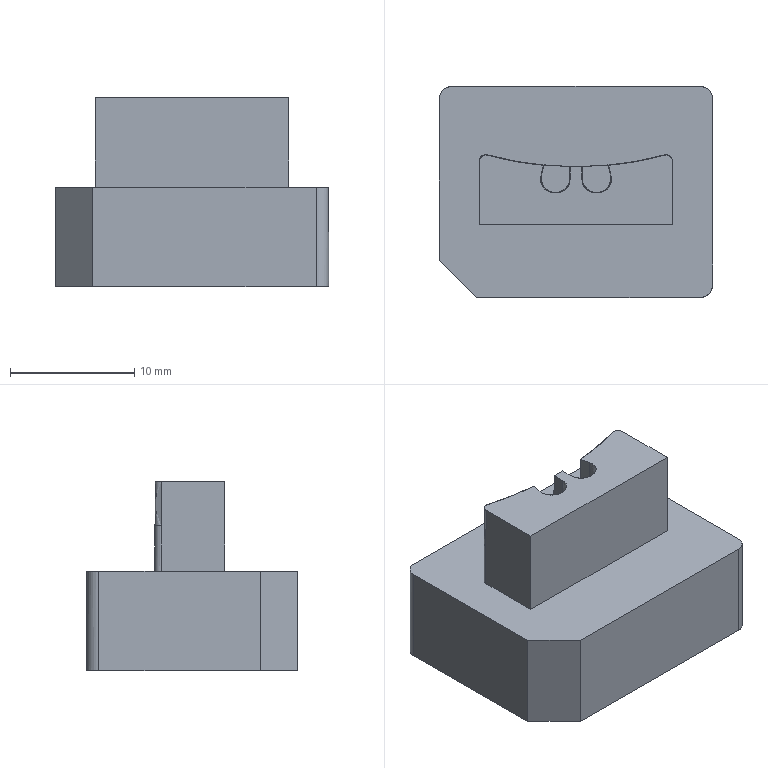NC program | PowerMill | posted by the shop | part box 22 x 17 x 15.232 mm
Lines 2761 to 5582 of 87032, first 2527 of 2822 lines:
( TOOL ID   D3C_1_1 )
( TOOL DIA. 3. TIP RAD 0 LENGTH 62.4 )
( Z = -7.32 )
T15 M6
T27
G91 G28 Z0
G0 G90 G54
M08
S18000 M3
X0 Y0 M8
G43 Z9.812 H15
X1.43 Y-5.074
Z.863
G1 Z-.337 F3000
X1.438 Y-5.057 F5000
G3 X1.361 Y-4.825 I-.155 J.077
G1 X0 Y-4.144
X-7.809
X-8.232 Y-4.074
X-8.399 Y-4.01
X-8.654 Y-3.864
X-8.949 Y-3.588
X-9.076 Y-3.409
X-9.194 Y-3.166
X-9.289 Y-2.744
X-9.294 Y-2.322
Y2.322
X-9.268 Y2.744
X-9.167 Y3.166
X-8.95 Y3.588
X-8.654 Y3.936
X-8.232 Y4.236
X-7.809 Y4.401
X-7.387 Y4.478
X-6.965 Y4.452
X-5.277 Y4.065
X-4.01 Y3.835
X-2.21 Y3.588
X-1.9 Y3.456
X-1.578 Y3.201
X-1.494 Y3.168
X-1.406 Y3.19
X-1.055 Y3.407
X-.633 Y3.515
X.633
X1.055 Y3.407
X1.406 Y3.19
X1.482 Y3.168
X1.558 Y3.189
X1.578 Y3.2
X1.9 Y3.456
X2.21 Y3.588
X3.588 Y3.775
X5.277 Y4.065
X6.826 Y4.432
X7.387 Y4.478
X7.693 Y4.432
X8.232 Y4.236
X8.569 Y4.01
X8.95 Y3.588
X9.162 Y3.166
X9.259 Y2.744
X9.294 Y2.322
Y-2.322
X9.289 Y-2.744
X9.194 Y-3.166
X9.076 Y-3.409
X8.949 Y-3.588
X8.654 Y-3.864
X8.399 Y-4.01
X8.232 Y-4.074
X7.809 Y-4.144
X0
X1.43 Y-5.074 Z-.485
X1.438 Y-5.057
G3 X1.361 Y-4.825 I-.155 J.077
G1 X0 Y-4.144
X-7.809
X-8.232 Y-4.074
X-8.399 Y-4.01
X-8.654 Y-3.864
X-8.949 Y-3.588
X-9.076 Y-3.409
X-9.194 Y-3.166
X-9.289 Y-2.744
X-9.294 Y-2.322
Y2.322
X-9.268 Y2.744
X-9.168 Y3.166
X-8.95 Y3.588
X-8.654 Y3.937
X-8.232 Y4.242
X-7.809 Y4.404
X-7.387 Y4.481
X-6.965 Y4.454
X-5.699 Y4.164
X-4.01 Y3.838
X-2.205 Y3.588
X-1.9 Y3.459
X-1.578 Y3.203
X-1.493 Y3.171
X-1.405 Y3.194
X-1.055 Y3.412
X-.633 Y3.52
X.633
X1.055 Y3.412
X1.405 Y3.194
X1.493 Y3.171
X1.578 Y3.203
X1.9 Y3.459
X2.205 Y3.588
X3.726 Y3.798
X3.728 Y3.799
X5.017 Y4.02
X5.277 Y4.067
X6.818 Y4.432
X7.387 Y4.481
X7.699 Y4.432
X8.232 Y4.242
X8.573 Y4.01
X8.95 Y3.588
X9.168 Y3.166
X9.261 Y2.744
X9.294 Y2.322
Y-2.322
X9.289 Y-2.744
X9.194 Y-3.166
X9.076 Y-3.409
X8.949 Y-3.588
X8.654 Y-3.864
X8.399 Y-4.01
X8.232 Y-4.074
X7.809 Y-4.144
X0
X1.43 Y-5.074 Z-.634
X1.438 Y-5.057
G3 X1.361 Y-4.825 I-.155 J.077
G1 X0 Y-4.144
X-7.809
X-8.232 Y-4.074
X-8.399 Y-4.01
X-8.654 Y-3.864
X-8.949 Y-3.588
X-9.076 Y-3.409
X-9.194 Y-3.166
X-9.289 Y-2.744
X-9.294 Y-2.322
Y2.322
X-9.268 Y2.744
X-9.168 Y3.166
X-8.95 Y3.588
X-8.654 Y3.938
X-8.232 Y4.243
X-7.809 Y4.408
X-7.387 Y4.483
X-6.965 Y4.456
X-5.699 Y4.165
X-4.01 Y3.839
X-2.322 Y3.619
X-2.265 Y3.597
X-2.205 Y3.588
X-1.955 Y3.483
X-1.9 Y3.462
X-1.578 Y3.206
X-1.493 Y3.174
X-1.405 Y3.196
X-1.055 Y3.416
X-.633 Y3.521
X.633
X1.055 Y3.416
X1.405 Y3.196
X1.493 Y3.174
X1.578 Y3.206
X1.9 Y3.462
X2.199 Y3.588
X3.772 Y3.806
X3.775 Y3.807
X4.862 Y3.994
X5.277 Y4.069
X6.812 Y4.432
X7.387 Y4.483
X7.703 Y4.432
X8.232 Y4.243
X8.574 Y4.01
X8.95 Y3.588
X9.168 Y3.166
X9.264 Y2.744
X9.294 Y2.322
Y-2.322
X9.289 Y-2.744
X9.194 Y-3.166
X9.076 Y-3.409
X8.949 Y-3.588
X8.654 Y-3.864
X8.399 Y-4.01
X8.232 Y-4.074
X7.809 Y-4.144
X0
X1.43 Y-5.074 Z-.782
X1.438 Y-5.057
G3 X1.361 Y-4.825 I-.155 J.077
G1 X0 Y-4.144
X-7.809
X-8.232 Y-4.074
X-8.399 Y-4.01
X-8.654 Y-3.864
X-8.949 Y-3.588
X-9.076 Y-3.409
X-9.194 Y-3.166
X-9.289 Y-2.744
X-9.294 Y-2.322
Y2.322
X-9.269 Y2.744
X-9.169 Y3.166
X-8.95 Y3.588
X-8.654 Y3.94
X-8.232 Y4.244
X-7.809 Y4.411
X-7.387 Y4.484
X-6.965 Y4.458
X-5.649 Y4.156
X-5.646 Y4.155
X-4.128 Y3.862
X-4.01 Y3.841
X-2.322 Y3.621
X-2.109 Y3.548
X-1.9 Y3.465
X-1.578 Y3.209
X-1.493 Y3.176
X-1.405 Y3.199
X-1.055 Y3.418
X-.633 Y3.523
X.633
X1.055 Y3.418
X1.405 Y3.199
X1.493 Y3.176
X1.578 Y3.209
X1.9 Y3.465
X2.194 Y3.588
X3.588 Y3.783
X5.277 Y4.07
X6.806 Y4.432
X7.387 Y4.484
X7.707 Y4.432
X8.232 Y4.244
X8.575 Y4.01
X8.95 Y3.588
X9.169 Y3.166
X9.266 Y2.744
X9.294 Y2.322
Y-2.322
X9.289 Y-2.744
X9.194 Y-3.166
X9.076 Y-3.409
X8.949 Y-3.588
X8.654 Y-3.864
X8.399 Y-4.01
X8.232 Y-4.074
X7.809 Y-4.144
X0
X1.43 Y-5.074 Z-.931
X1.438 Y-5.057
G3 X1.361 Y-4.825 I-.155 J.077
G1 X0 Y-4.144
X-7.809
X-8.232 Y-4.074
X-8.399 Y-4.01
X-8.654 Y-3.864
X-8.949 Y-3.588
X-9.076 Y-3.409
X-9.194 Y-3.166
X-9.289 Y-2.744
X-9.294 Y-2.322
Y2.322
X-9.269 Y2.744
X-9.169 Y3.166
X-8.95 Y3.588
X-8.654 Y3.941
X-8.232 Y4.246
X-7.809 Y4.412
X-7.387 Y4.486
X-6.965 Y4.46
X-5.608 Y4.148
X-4.246 Y3.885
X-4.01 Y3.842
X-2.322 Y3.622
X-2.244 Y3.593
X-2.205 Y3.588
X-2.054 Y3.524
X-1.9 Y3.467
X-1.577 Y3.211
X-1.493 Y3.179
X-1.405 Y3.201
X-1.055 Y3.419
X-.633 Y3.524
X.633
X1.055 Y3.419
X1.405 Y3.201
X1.492 Y3.179
X1.577 Y3.211
X1.9 Y3.467
X1.949 Y3.485
X1.952 Y3.487
X2.194 Y3.588
X2.26 Y3.598
X2.322 Y3.622
X3.588 Y3.784
X5.277 Y4.071
X6.8 Y4.432
X7.387 Y4.486
X7.71 Y4.432
X8.232 Y4.246
X8.576 Y4.01
X8.951 Y3.588
X9.169 Y3.166
X9.269 Y2.744
X9.294 Y2.322
Y-2.322
X9.289 Y-2.744
X9.194 Y-3.166
X9.076 Y-3.409
X8.949 Y-3.588
X8.654 Y-3.864
X8.399 Y-4.01
X8.232 Y-4.074
X7.809 Y-4.144
X0
X1.43 Y-5.074 Z-1.079
X1.438 Y-5.057
G3 X1.361 Y-4.825 I-.155 J.077
G1 X0 Y-4.144
X-7.809
X-8.232 Y-4.074
X-8.399 Y-4.01
X-8.654 Y-3.864
X-8.949 Y-3.588
X-9.076 Y-3.409
X-9.194 Y-3.166
X-9.289 Y-2.744
X-9.294 Y-2.322
Y2.322
X-9.269 Y2.744
X-9.17 Y3.166
X-8.951 Y3.588
X-8.654 Y3.943
X-8.232 Y4.247
X-7.809 Y4.412
X-7.387 Y4.487
X-6.965 Y4.462
X-5.568 Y4.14
X-4.79 Y3.987
X-4.01 Y3.844
X-2.322 Y3.624
X-2.236 Y3.592
X-2.205 Y3.588
X-2.054 Y3.525
X-1.9 Y3.469
X-1.577 Y3.214
X-1.492 Y3.182
X-1.405 Y3.204
X-1.055 Y3.421
X-.633 Y3.526
X.633
X1.055 Y3.421
X1.405 Y3.204
X1.492 Y3.181
X1.577 Y3.214
X1.9 Y3.469
X1.986 Y3.501
X2.194 Y3.588
X2.244 Y3.595
X2.258 Y3.6
X2.322 Y3.624
X3.588 Y3.785
X5.277 Y4.073
X6.795 Y4.432
X7.387 Y4.487
X7.714 Y4.432
X8.232 Y4.247
X8.577 Y4.01
X8.951 Y3.588
X9.17 Y3.166
X9.269 Y2.744
X9.294 Y2.322
Y-2.322
X9.289 Y-2.744
X9.194 Y-3.166
X9.076 Y-3.409
X8.949 Y-3.588
X8.654 Y-3.864
X8.399 Y-4.01
X8.232 Y-4.074
X7.809 Y-4.144
X0
X1.43 Y-5.074 Z-1.228
X1.438 Y-5.057
G3 X1.361 Y-4.825 I-.155 J.077
G1 X0 Y-4.144
X-7.809
X-8.232 Y-4.074
X-8.399 Y-4.01
X-8.654 Y-3.864
X-8.949 Y-3.588
X-9.076 Y-3.409
X-9.194 Y-3.166
X-9.289 Y-2.744
X-9.294 Y-2.322
Y2.322
X-9.269 Y2.744
X-9.17 Y3.166
X-8.951 Y3.588
X-8.654 Y3.944
X-8.232 Y4.248
X-7.809 Y4.413
X-7.387 Y4.488
X-6.965 Y4.464
X-5.531 Y4.133
X-4.771 Y3.984
X-4.01 Y3.845
X-2.322 Y3.625
X-2.229 Y3.591
X-2.205 Y3.588
X-2.054 Y3.526
X-1.9 Y3.471
X-1.577 Y3.216
X-1.492 Y3.184
X-1.405 Y3.206
X-1.055 Y3.423
X-.633 Y3.527
X.633
X1.055 Y3.423
X1.405 Y3.206
X1.492 Y3.184
X1.577 Y3.216
X1.9 Y3.471
X2.048 Y3.526
X2.194 Y3.588
X2.236 Y3.594
X2.251 Y3.599
X2.322 Y3.625
X3.588 Y3.787
X5.277 Y4.074
X6.789 Y4.432
X7.387 Y4.488
X7.72 Y4.432
X8.232 Y4.248
X8.578 Y4.01
X8.951 Y3.588
X9.17 Y3.166
X9.27 Y2.744
X9.294 Y2.322
Y-2.322
X9.289 Y-2.744
X9.194 Y-3.166
X9.076 Y-3.409
X8.949 Y-3.588
X8.654 Y-3.864
X8.399 Y-4.01
X8.232 Y-4.074
X7.809 Y-4.144
X0
X1.43 Y-5.074 Z-1.377
X1.438 Y-5.057
G3 X1.361 Y-4.825 I-.155 J.077
G1 X0 Y-4.144
X-7.809
X-8.232 Y-4.074
X-8.399 Y-4.01
X-8.654 Y-3.864
X-8.949 Y-3.588
X-9.076 Y-3.409
X-9.194 Y-3.166
X-9.289 Y-2.744
X-9.294 Y-2.322
Y2.322
X-9.269 Y2.744
X-9.171 Y3.166
X-8.951 Y3.588
X-8.654 Y3.945
X-8.232 Y4.25
X-7.809 Y4.414
X-7.387 Y4.49
X-6.965 Y4.465
X-5.495 Y4.126
X-4.753 Y3.982
X-4.01 Y3.846
X-2.322 Y3.626
X-2.222 Y3.59
X-2.205 Y3.588
X-2.141 Y3.561
X-1.9 Y3.473
X-1.576 Y3.218
X-1.492 Y3.186
X-1.404 Y3.209
X-1.055 Y3.425
X-.633 Y3.528
X.633
X1.055 Y3.425
X1.404 Y3.209
X1.492 Y3.187
X1.576 Y3.218
X1.9 Y3.473
X2.048 Y3.527
X2.194 Y3.588
X2.229 Y3.593
X2.244 Y3.598
X2.322 Y3.626
X3.588 Y3.788
X5.277 Y4.075
X6.119 Y4.277
X6.965 Y4.465
X7.387 Y4.49
X7.725 Y4.432
X8.232 Y4.25
X8.579 Y4.01
X8.951 Y3.588
X9.171 Y3.166
X9.27 Y2.744
X9.294 Y2.322
Y-2.322
X9.289 Y-2.744
X9.194 Y-3.166
X9.076 Y-3.409
X8.949 Y-3.588
X8.654 Y-3.864
X8.399 Y-4.01
X8.232 Y-4.074
X7.809 Y-4.144
X0
X1.43 Y-5.074 Z-1.525
X1.438 Y-5.057
G3 X1.361 Y-4.825 I-.155 J.077
G1 X0 Y-4.144
X-7.809
X-8.232 Y-4.074
X-8.399 Y-4.01
X-8.654 Y-3.864
X-8.949 Y-3.588
X-9.076 Y-3.409
X-9.194 Y-3.166
X-9.289 Y-2.744
X-9.294 Y-2.322
Y2.322
X-9.269 Y2.744
X-9.171 Y3.166
X-8.951 Y3.588
X-8.654 Y3.947
X-8.232 Y4.251
X-7.809 Y4.415
X-7.387 Y4.491
X-6.965 Y4.467
X-5.459 Y4.119
X-4.735 Y3.979
X-4.01 Y3.848
X-2.322 Y3.628
X-2.168 Y3.588
X-1.9 Y3.475
X-1.576 Y3.221
X-1.492 Y3.189
X-1.405 Y3.211
X-1.055 Y3.427
X-.633 Y3.53
X.633
X1.055 Y3.427
X1.404 Y3.211
X1.492 Y3.189
X1.576 Y3.221
X1.9 Y3.475
X2.167 Y3.588
X2.322 Y3.628
X3.588 Y3.789
X5.277 Y4.077
X5.727 Y4.181
X6.789 Y4.432
X6.836 Y4.437
X6.845 Y4.439
X6.965 Y4.467
X7.387 Y4.491
X7.731 Y4.432
X8.232 Y4.251
X8.58 Y4.01
X8.951 Y3.588
X9.171 Y3.166
X9.27 Y2.744
X9.294 Y2.322
Y-2.322
X9.289 Y-2.744
X9.194 Y-3.166
X9.076 Y-3.409
X8.949 Y-3.588
X8.654 Y-3.864
X8.399 Y-4.01
X8.232 Y-4.074
X7.809 Y-4.144
X0
X1.43 Y-5.074 Z-1.674
X1.438 Y-5.057
G3 X1.361 Y-4.825 I-.155 J.077
G1 X0 Y-4.144
X-7.809
X-8.232 Y-4.074
X-8.399 Y-4.01
X-8.654 Y-3.864
X-8.949 Y-3.588
X-9.076 Y-3.409
X-9.194 Y-3.166
X-9.289 Y-2.744
X-9.294 Y-2.322
Y2.322
X-9.27 Y2.744
X-9.172 Y3.166
X-8.951 Y3.588
X-8.654 Y3.948
X-8.232 Y4.252
X-7.809 Y4.416
X-7.387 Y4.492
X-6.965 Y4.468
X-5.423 Y4.112
X-4.717 Y3.976
X-4.01 Y3.849
X-2.322 Y3.629
X-2.162 Y3.588
X-1.9 Y3.477
X-1.576 Y3.223
X-1.492 Y3.192
X-1.404 Y3.214
X-1.055 Y3.429
X-.633 Y3.531
X.633
X1.055 Y3.429
X1.404 Y3.214
X1.491 Y3.192
X1.576 Y3.223
X1.9 Y3.477
X2.162 Y3.588
X2.322 Y3.629
X3.588 Y3.791
X5.277 Y4.078
X5.954 Y4.234
X6.789 Y4.432
X6.826 Y4.436
X6.835 Y4.438
X6.965 Y4.468
X7.387 Y4.492
X7.736 Y4.432
X8.232 Y4.252
X8.581 Y4.01
X8.951 Y3.588
X9.172 Y3.166
X9.27 Y2.744
X9.294 Y2.322
Y-2.322
X9.289 Y-2.744
X9.194 Y-3.166
X9.076 Y-3.409
X8.949 Y-3.588
X8.654 Y-3.864
X8.399 Y-4.01
X8.232 Y-4.074
X7.809 Y-4.144
X0
X1.43 Y-5.074 Z-1.822
X1.438 Y-5.057
G3 X1.361 Y-4.825 I-.155 J.077
G1 X0 Y-4.144
X-7.809
X-8.232 Y-4.074
X-8.399 Y-4.01
X-8.654 Y-3.864
X-8.949 Y-3.588
X-9.076 Y-3.409
X-9.194 Y-3.166
X-9.289 Y-2.744
X-9.294 Y-2.322
Y2.322
X-9.27 Y2.744
X-9.172 Y3.166
X-8.951 Y3.588
X-8.654 Y3.949
X-8.232 Y4.254
X-7.809 Y4.416
X-7.387 Y4.494
X-6.965 Y4.469
X-5.387 Y4.105
X-4.699 Y3.973
X-4.01 Y3.85
X-2.322 Y3.631
X-2.157 Y3.588
X-1.9 Y3.479
X-1.575 Y3.226
X-1.491 Y3.194
X-1.404 Y3.216
X-1.055 Y3.43
X-.633 Y3.533
X.633
X1.055 Y3.43
X1.404 Y3.216
X1.491 Y3.194
X1.575 Y3.226
X1.9 Y3.479
X2.157 Y3.588
X2.322 Y3.631
X3.588 Y3.792
X5.277 Y4.079
X6.182 Y4.288
X6.789 Y4.432
X6.816 Y4.435
X6.825 Y4.437
X6.965 Y4.469
X7.387 Y4.494
X7.742 Y4.432
X8.232 Y4.254
X8.582 Y4.01
X8.951 Y3.588
X9.172 Y3.166
X9.27 Y2.744
X9.294 Y2.322
Y-2.322
X9.289 Y-2.744
X9.194 Y-3.166
X9.076 Y-3.409
X8.949 Y-3.588
X8.654 Y-3.864
X8.399 Y-4.01
X8.232 Y-4.074
X7.809 Y-4.144
X0
X1.43 Y-5.074 Z-1.971
X1.438 Y-5.057
G3 X1.361 Y-4.825 I-.155 J.077
G1 X0 Y-4.144
X-7.809
X-8.232 Y-4.074
X-8.399 Y-4.01
X-8.654 Y-3.864
X-8.949 Y-3.588
X-9.076 Y-3.409
X-9.194 Y-3.166
X-9.289 Y-2.744
X-9.294 Y-2.322
Y2.322
X-9.27 Y2.744
X-9.173 Y3.166
X-8.952 Y3.588
X-8.654 Y3.951
X-8.232 Y4.255
X-7.809 Y4.418
X-7.387 Y4.495
X-6.965 Y4.471
X-5.351 Y4.098
X-5.043 Y4.038
X-4.01 Y3.852
X-2.322 Y3.632
X-2.152 Y3.588
X-1.9 Y3.481
X-1.69 Y3.346
X-1.577 Y3.241
G3 X-1.397 Y3.224 I.102 J.11
G1 X-1.055 Y3.432
X-.633 Y3.534
X.633
X1.055 Y3.432
X1.404 Y3.218
X1.491 Y3.197
X1.575 Y3.228
X1.9 Y3.481
X2.152 Y3.588
X2.322 Y3.632
X3.588 Y3.793
X5.277 Y4.081
X6.411 Y4.343
X6.789 Y4.432
X6.806 Y4.434
X6.815 Y4.436
X6.965 Y4.471
X7.387 Y4.495
X7.747 Y4.432
X8.232 Y4.255
X8.583 Y4.01
X8.952 Y3.588
X9.173 Y3.166
X9.271 Y2.744
X9.294 Y2.322
Y-2.322
X9.289 Y-2.744
X9.194 Y-3.166
X9.076 Y-3.409
X8.949 Y-3.588
X8.654 Y-3.864
X8.399 Y-4.01
X8.232 Y-4.074
X7.809 Y-4.144
X0
X1.43 Y-5.074 Z-2.12
X1.438 Y-5.057
G3 X1.361 Y-4.825 I-.155 J.077
G1 X0 Y-4.144
X-7.809
X-8.232 Y-4.074
X-8.399 Y-4.01
X-8.654 Y-3.864
X-8.949 Y-3.588
X-9.076 Y-3.409
X-9.194 Y-3.166
X-9.289 Y-2.744
X-9.294 Y-2.322
Y2.322
X-9.27 Y2.744
X-9.173 Y3.166
X-8.954 Y3.588
X-8.654 Y3.952
X-8.232 Y4.256
X-7.809 Y4.42
X-7.387 Y4.496
X-6.965 Y4.472
X-5.315 Y4.091
X-5.156 Y4.06
X-4.01 Y3.853
X-2.322 Y3.634
X-2.146 Y3.588
X-1.9 Y3.483
X-1.69 Y3.348
X-1.576 Y3.243
G3 X-1.396 Y3.226 I.101 J.11
G1 X-1.055 Y3.434
X-.633 Y3.536
X.633
X1.055 Y3.434
X1.392 Y3.229
G3 X1.586 Y3.26 I.078 J.13
G1 X1.9 Y3.483
X2.147 Y3.588
X2.322 Y3.634
X3.588 Y3.795
X5.277 Y4.082
X6.642 Y4.397
X6.789 Y4.432
X6.797 Y4.433
X6.805 Y4.435
X6.965 Y4.472
X7.387 Y4.496
X7.753 Y4.432
X8.232 Y4.256
X8.584 Y4.01
X8.953 Y3.588
X9.173 Y3.166
X9.271 Y2.744
X9.294 Y2.322
Y-2.322
X9.289 Y-2.744
X9.194 Y-3.166
X9.076 Y-3.409
X8.949 Y-3.588
X8.654 Y-3.864
X8.399 Y-4.01
X8.232 Y-4.074
X7.809 Y-4.144
X0
X1.43 Y-5.074 Z-2.268
X1.438 Y-5.057
G3 X1.361 Y-4.825 I-.155 J.077
G1 X0 Y-4.144
X-7.809
X-8.232 Y-4.074
X-8.399 Y-4.01
X-8.654 Y-3.864
X-8.949 Y-3.588
X-9.076 Y-3.409
X-9.194 Y-3.166
X-9.289 Y-2.744
X-9.294 Y-2.322
Y2.322
X-9.271 Y2.744
X-9.174 Y3.166
X-8.955 Y3.588
X-8.654 Y3.953
X-8.232 Y4.258
X-7.809 Y4.422
X-7.387 Y4.498
X-6.965 Y4.473
X-5.279 Y4.084
X-5.269 Y4.082
X-4.01 Y3.854
X-2.322 Y3.635
X-2.141 Y3.588
X-1.9 Y3.485
X-1.69 Y3.351
X-1.577 Y3.247
X-1.49 Y3.208
X-1.398 Y3.229
X-1.055 Y3.436
X-.633 Y3.537
X.633
X1.055 Y3.436
X1.392 Y3.231
G3 X1.586 Y3.263 I.078 J.13
G1 X1.9 Y3.485
X2.142 Y3.588
X2.322 Y3.635
X3.588 Y3.796
X5.277 Y4.083
X5.281 Y4.084
X6.965 Y4.473
X7.387 Y4.498
X7.759 Y4.432
X8.232 Y4.258
X8.586 Y4.01
X8.955 Y3.588
X9.174 Y3.166
X9.271 Y2.744
X9.294 Y2.322
Y-2.322
X9.289 Y-2.744
X9.194 Y-3.166
X9.076 Y-3.409
X8.949 Y-3.588
X8.654 Y-3.864
X8.399 Y-4.01
X8.232 Y-4.074
X7.809 Y-4.144
X0
X1.43 Y-5.074 Z-2.417
X1.438 Y-5.057
G3 X1.361 Y-4.825 I-.155 J.077
G1 X0 Y-4.144
X-7.809
X-8.232 Y-4.074
X-8.399 Y-4.01
X-8.654 Y-3.864
X-8.949 Y-3.588
X-9.076 Y-3.409
X-9.194 Y-3.166
X-9.289 Y-2.744
X-9.294 Y-2.322
Y2.322
X-9.271 Y2.744
X-9.174 Y3.166
X-8.957 Y3.588
X-8.654 Y3.954
X-8.232 Y4.259
X-7.809 Y4.424
X-7.387 Y4.499
X-6.965 Y4.475
X-5.277 Y4.084
X-4.01 Y3.855
X-2.322 Y3.637
X-2.136 Y3.588
X-1.9 Y3.487
X-1.69 Y3.353
X-1.576 Y3.248
G3 X-1.387 Y3.237 I.102 J.112
G1 X-1.055 Y3.438
X-.633 Y3.539
X.633
X1.055 Y3.438
X1.392 Y3.233
G3 X1.586 Y3.266 I.078 J.13
G1 X1.9 Y3.487
X2.137 Y3.588
X2.322 Y3.637
X3.588 Y3.797
X5.277 Y4.085
X6.965 Y4.475
X7.387 Y4.499
X7.764 Y4.432
X8.232 Y4.259
X8.587 Y4.01
X8.957 Y3.588
X9.174 Y3.166
X9.271 Y2.744
X9.294 Y2.322
Y-2.322
X9.289 Y-2.744
X9.194 Y-3.166
X9.076 Y-3.409
X8.949 Y-3.588
X8.654 Y-3.864
X8.399 Y-4.01
X8.232 Y-4.074
X7.809 Y-4.144
X0
X1.43 Y-5.074 Z-2.565
X1.438 Y-5.057
G3 X1.361 Y-4.825 I-.155 J.077
G1 X0 Y-4.144
X-7.809
X-8.232 Y-4.074
X-8.399 Y-4.01
X-8.654 Y-3.864
X-8.949 Y-3.588
X-9.076 Y-3.409
X-9.194 Y-3.166
X-9.289 Y-2.744
X-9.294 Y-2.322
Y2.322
X-9.271 Y2.744
X-9.175 Y3.166
X-8.958 Y3.588
X-8.654 Y3.956
X-8.232 Y4.26
X-7.809 Y4.426
X-7.387 Y4.5
X-6.965 Y4.476
X-5.277 Y4.086
X-4.01 Y3.857
X-2.322 Y3.638
X-2.131 Y3.588
X-1.9 Y3.489
X-1.69 Y3.355
X-1.575 Y3.25
G3 X-1.386 Y3.239 I.101 J.112
G1 X-1.055 Y3.44
X-.633 Y3.54
X.633
X1.055 Y3.44
X1.392 Y3.236
G3 X1.586 Y3.269 I.078 J.131
G1 X1.9 Y3.489
X2.132 Y3.588
X2.322 Y3.638
X3.588 Y3.798
X5.277 Y4.086
X6.965 Y4.476
X7.387 Y4.5
X7.77 Y4.432
X8.232 Y4.26
X8.589 Y4.01
X8.958 Y3.588
X9.175 Y3.166
X9.271 Y2.744
X9.294 Y2.322
Y-2.322
X9.289 Y-2.744
X9.194 Y-3.166
X9.076 Y-3.409
X8.949 Y-3.588
X8.654 Y-3.864
X8.399 Y-4.01
X8.232 Y-4.074
X7.809 Y-4.144
X0
X1.43 Y-5.074 Z-2.714
X1.438 Y-5.057
G3 X1.361 Y-4.825 I-.155 J.077
G1 X0 Y-4.144
X-7.809
X-8.232 Y-4.074
X-8.399 Y-4.01
X-8.654 Y-3.864
X-8.949 Y-3.588
X-9.076 Y-3.409
X-9.194 Y-3.166
X-9.289 Y-2.744
X-9.294 Y-2.322
Y2.322
X-9.271 Y2.744
X-9.175 Y3.166
X-8.96 Y3.588
X-8.654 Y3.957
X-8.232 Y4.262
X-7.809 Y4.427
X-7.387 Y4.502
X-6.965 Y4.477
X-5.277 Y4.087
X-4.01 Y3.858
X-2.322 Y3.64
X-2.126 Y3.588
X-1.9 Y3.491
X-1.69 Y3.358
X-1.575 Y3.253
X-1.488 Y3.214
X-1.396 Y3.235
X-1.055 Y3.441
X-.633 Y3.541
X.633
X1.055 Y3.441
X1.392 Y3.238
G3 X1.587 Y3.271 I.078 J.131
G1 X1.9 Y3.491
X2.127 Y3.588
X2.322 Y3.64
X3.588 Y3.8
X5.277 Y4.087
X6.965 Y4.477
X7.387 Y4.502
X7.62 Y4.459
X7.77 Y4.432
X7.777 Y4.43
X7.785 Y4.429
X7.809 Y4.424
X8.232 Y4.262
X8.591 Y4.01
X8.96 Y3.588
X9.175 Y3.166
X9.272 Y2.744
X9.294 Y2.322
Y-2.322
X9.289 Y-2.744
X9.194 Y-3.166
X9.076 Y-3.409
X8.949 Y-3.588
X8.654 Y-3.864
X8.399 Y-4.01
X8.232 Y-4.074
X7.809 Y-4.144
X0
X1.43 Y-5.074 Z-2.862
X1.438 Y-5.057
G3 X1.361 Y-4.825 I-.155 J.077
G1 X0 Y-4.144
X-7.809
X-8.232 Y-4.074
X-8.399 Y-4.01
X-8.654 Y-3.864
X-8.949 Y-3.588
X-9.076 Y-3.409
X-9.194 Y-3.166
X-9.289 Y-2.744
X-9.294 Y-2.322
Y2.322
X-9.272 Y2.744
X-9.176 Y3.166
X-8.962 Y3.588
X-8.654 Y3.958
X-8.232 Y4.263
X-7.809 Y4.429
X-7.387 Y4.503
X-6.965 Y4.479
X-5.277 Y4.088
X-4.01 Y3.859
X-2.322 Y3.641
X-2.121 Y3.588
X-1.9 Y3.493
X-1.69 Y3.36
X-1.575 Y3.256
G3 X-1.388 Y3.245 I.101 J.112
G1 X-1.055 Y3.443
X-.633 Y3.543
X.633
X1.055 Y3.443
X1.392 Y3.24
G3 X1.587 Y3.274 I.078 J.131
G1 X1.9 Y3.493
X2.122 Y3.588
X2.322 Y3.641
X3.588 Y3.801
X5.277 Y4.088
X6.965 Y4.479
X7.387 Y4.503
X7.809 Y4.425
X8.232 Y4.263
X8.592 Y4.01
X8.962 Y3.588
X9.176 Y3.166
X9.272 Y2.744
X9.294 Y2.322
Y-2.322
X9.289 Y-2.744
X9.194 Y-3.166
X9.076 Y-3.409
X8.949 Y-3.588
X8.654 Y-3.864
X8.399 Y-4.01
X8.232 Y-4.074
X7.809 Y-4.144
X0
X1.43 Y-5.074 Z-3.011
X1.438 Y-5.057
G3 X1.361 Y-4.825 I-.155 J.077
G1 X0 Y-4.144
X-7.809
X-8.232 Y-4.074
X-8.399 Y-4.01
X-8.654 Y-3.864
X-8.949 Y-3.588
X-9.076 Y-3.409
X-9.194 Y-3.166
X-9.289 Y-2.744
X-9.294 Y-2.322
Y2.322
X-9.272 Y2.744
X-9.176 Y3.166
X-8.963 Y3.588
X-8.654 Y3.96
X-8.232 Y4.264
X-7.809 Y4.431
X-7.387 Y4.504
X-6.965 Y4.48
X-5.277 Y4.09
X-4.01 Y3.861
X-2.322 Y3.643
X-2.116 Y3.588
X-1.9 Y3.495
X-1.69 Y3.363
X-1.575 Y3.258
G3 X-1.387 Y3.247 I.101 J.113
G1 X-1.055 Y3.445
X-.633 Y3.544
X.633
X1.055 Y3.445
X1.391 Y3.243
G3 X1.587 Y3.277 I.078 J.131
G1 X1.9 Y3.495
X2.117 Y3.588
X2.322 Y3.643
X3.588 Y3.802
X5.277 Y4.09
X6.965 Y4.48
X7.387 Y4.504
X7.809 Y4.427
X8.232 Y4.264
X8.594 Y4.01
X8.963 Y3.588
X9.176 Y3.166
X9.272 Y2.744
X9.294 Y2.322
Y-2.322
X9.289 Y-2.744
X9.194 Y-3.166
X9.076 Y-3.409
X8.949 Y-3.588
X8.654 Y-3.864
X8.399 Y-4.01
X8.232 Y-4.074
X7.809 Y-4.144
X0
X1.43 Y-5.074 Z-3.16
X1.438 Y-5.057
G3 X1.361 Y-4.825 I-.155 J.077
G1 X0 Y-4.144
X-7.809
X-8.232 Y-4.074
X-8.399 Y-4.01
X-8.654 Y-3.864
X-8.949 Y-3.588
X-9.076 Y-3.409
X-9.194 Y-3.166
X-9.289 Y-2.744
X-9.294 Y-2.322
Y2.322
X-9.272 Y2.744
X-9.177 Y3.166
X-8.965 Y3.588
X-8.654 Y3.961
X-8.232 Y4.266
X-7.811 Y4.432
X-7.387 Y4.506
X-6.965 Y4.481
X-5.277 Y4.091
X-4.01 Y3.862
X-2.322 Y3.644
X-2.111 Y3.588
X-1.9 Y3.497
X-1.69 Y3.365
X-1.574 Y3.26
G3 X-1.386 Y3.248 I.101 J.113
G1 X-1.055 Y3.447
X-.633 Y3.546
X.633
X1.055 Y3.447
X1.391 Y3.245
G3 X1.587 Y3.28 I.078 J.132
G1 X1.9 Y3.497
X2.112 Y3.588
X2.322 Y3.644
X3.588 Y3.804
X5.277 Y4.091
X6.965 Y4.481
X7.387 Y4.506
X7.809 Y4.428
X8.232 Y4.266
X8.596 Y4.01
X8.965 Y3.588
X9.177 Y3.166
X9.272 Y2.744
X9.294 Y2.322
Y-2.322
X9.289 Y-2.744
X9.194 Y-3.166
X9.076 Y-3.409
X8.949 Y-3.588
X8.654 Y-3.864
X8.399 Y-4.01
X8.232 Y-4.074
X7.809 Y-4.144
X0
X1.43 Y-5.074 Z-3.308
X1.438 Y-5.057
G3 X1.361 Y-4.825 I-.155 J.077
G1 X0 Y-4.144
X-7.809
X-8.232 Y-4.074
X-8.399 Y-4.01
X-8.654 Y-3.864
X-8.949 Y-3.588
X-9.076 Y-3.409
X-9.194 Y-3.166
X-9.289 Y-2.744
X-9.294 Y-2.322
Y2.322
X-9.272 Y2.744
X-9.177 Y3.166
X-8.966 Y3.588
X-8.654 Y3.962
X-8.232 Y4.267
X-7.818 Y4.432
X-7.387 Y4.507
X-6.965 Y4.483
X-5.277 Y4.092
X-4.01 Y3.863
X-2.322 Y3.645
X-2.106 Y3.588
X-1.9 Y3.499
X-1.69 Y3.367
X-1.573 Y3.262
X-1.488 Y3.224
X-1.396 Y3.245
X-1.055 Y3.449
X-.633 Y3.547
X.633
X1.055 Y3.449
X1.391 Y3.247
G3 X1.587 Y3.282 I.077 J.132
G1 X1.9 Y3.499
X2.106 Y3.588
X2.322 Y3.645
X3.588 Y3.805
X5.277 Y4.092
X6.965 Y4.483
X7.387 Y4.507
X7.797 Y4.432
X7.808 Y4.428
X7.809
X7.878 Y4.402
X8.232 Y4.267
X8.597 Y4.01
X8.966 Y3.588
X9.177 Y3.166
X9.272 Y2.744
X9.294 Y2.322
Y-2.322
X9.289 Y-2.744
X9.194 Y-3.166
X9.076 Y-3.409
X8.949 Y-3.588
X8.654 Y-3.864
X8.399 Y-4.01
X8.232 Y-4.074
X7.809 Y-4.144
X0
X1.43 Y-5.074 Z-3.457
X1.438 Y-5.057
G3 X1.361 Y-4.825 I-.155 J.077
G1 X0 Y-4.144
X-7.809
X-8.232 Y-4.074
X-8.399 Y-4.01
X-8.654 Y-3.864
X-8.949 Y-3.588
X-9.076 Y-3.409
X-9.194 Y-3.166
X-9.289 Y-2.744
X-9.294 Y-2.322
Y2.322
X-9.273 Y2.744
X-9.178 Y3.166
X-8.968 Y3.588
X-8.654 Y3.964
X-8.232 Y4.268
X-7.825 Y4.432
X-7.387 Y4.508
X-6.965 Y4.484
X-5.277 Y4.094
X-4.01 Y3.865
X-2.322 Y3.647
X-2.101 Y3.588
X-1.9 Y3.501
X-1.691 Y3.37
X-1.574 Y3.265
G3 X-1.388 Y3.254 I.101 J.113
G1 X-1.055 Y3.451
X-.633 Y3.549
X.633
X1.055 Y3.451
X1.391 Y3.25
G3 X1.588 Y3.285 I.077 J.132
G1 X1.9 Y3.501
X2.101 Y3.588
X2.322 Y3.647
X3.588 Y3.806
X5.277 Y4.094
X6.965 Y4.484
X7.387 Y4.508
X7.803 Y4.432
X8.232 Y4.268
X8.599 Y4.01
X8.968 Y3.588
X9.178 Y3.166
X9.273 Y2.744
X9.294 Y2.322
Y-2.322
X9.289 Y-2.744
X9.194 Y-3.166
X9.076 Y-3.409
X8.949 Y-3.588
X8.654 Y-3.864
X8.399 Y-4.01
X8.232 Y-4.074
X7.809 Y-4.144
X0
X1.43 Y-5.074 Z-3.605
X1.438 Y-5.057
G3 X1.361 Y-4.825 I-.155 J.077
G1 X0 Y-4.144
X-7.809
X-8.232 Y-4.074
X-8.399 Y-4.01
X-8.654 Y-3.864
X-8.949 Y-3.588
X-9.076 Y-3.409
X-9.194 Y-3.166
X-9.289 Y-2.744
X-9.294 Y-2.322
Y2.322
X-9.273 Y2.744
X-9.178 Y3.166
X-8.97 Y3.588
X-8.654 Y3.965
X-8.232 Y4.27
X-7.831 Y4.432
X-7.387 Y4.51
X-6.965 Y4.485
X-5.277 Y4.095
X-4.01 Y3.868
X-2.322 Y3.648
X-2.096 Y3.588
X-1.9 Y3.503
X-1.691 Y3.372
X-1.573 Y3.267
G3 X-1.387 Y3.256 I.1 J.113
G1 X-1.055 Y3.452
X-.633 Y3.55
X.633
X1.055 Y3.452
X1.391 Y3.252
G3 X1.588 Y3.288 I.077 J.132
G1 X1.9 Y3.503
X2.096 Y3.588
X2.322 Y3.648
X3.588 Y3.808
X5.277 Y4.095
X6.965 Y4.485
X7.387 Y4.51
X7.809 Y4.432
X8.232 Y4.27
X8.602 Y4.01
X8.97 Y3.588
X9.178 Y3.166
X9.273 Y2.744
X9.294 Y2.322
Y-2.322
X9.289 Y-2.744
X9.194 Y-3.166
X9.076 Y-3.409
X8.949 Y-3.588
X8.654 Y-3.864
X8.399 Y-4.01
X8.232 Y-4.074
X7.809 Y-4.144
X0
X1.43 Y-5.074 Z-3.754
X1.438 Y-5.057
G3 X1.361 Y-4.825 I-.155 J.077
G1 X0 Y-4.144
X-7.809
X-8.232 Y-4.074
X-8.399 Y-4.01
X-8.654 Y-3.864
X-8.949 Y-3.588
X-9.076 Y-3.409
X-9.194 Y-3.166
X-9.289 Y-2.744
X-9.294 Y-2.322
Y2.322
X-9.273 Y2.744
X-9.179 Y3.166
X-8.971 Y3.588
X-8.654 Y3.967
X-8.232 Y4.271
X-7.838 Y4.432
X-7.387 Y4.511
X-6.965 Y4.487
X-5.277 Y4.1
X-3.683 Y3.825
X-3.409 Y3.79
X-1.9 Y3.627
X-.211 Y3.559
X1.477 Y3.601
X3.166 Y3.757
X4.565 Y3.974
X4.872 Y4.026
X4.875 Y4.027
X6.965 Y4.487
X7.387 Y4.511
X7.836 Y4.432
X8.232 Y4.271
X8.606 Y4.01
X8.971 Y3.588
X9.179 Y3.166
X9.273 Y2.744
X9.294 Y2.322
Y-2.322
X9.289 Y-2.744
X9.194 Y-3.166
X9.076 Y-3.409
X8.949 Y-3.588
X8.654 Y-3.864
X8.399 Y-4.01
X8.232 Y-4.074
X7.809 Y-4.144
X0
X1.43 Y-5.074 Z-3.903
X1.438 Y-5.057
G3 X1.361 Y-4.825 I-.155 J.077
G1 X0 Y-4.144
X-7.809
X-8.232 Y-4.074
X-8.399 Y-4.01
X-8.654 Y-3.864
X-8.949 Y-3.588
X-9.076 Y-3.409
X-9.194 Y-3.166
X-9.289 Y-2.744
X-9.294 Y-2.322
Y2.322
X-9.273 Y2.744
X-9.179 Y3.166
X-8.971 Y3.588
X-8.654 Y3.967
X-8.232 Y4.271
X-7.838 Y4.432
X-7.387 Y4.511
X-6.965 Y4.487
X-5.277 Y4.101
X-3.68 Y3.825
X-3.417 Y3.791
X-1.9 Y3.628
X-.211 Y3.56
X1.477 Y3.601
X3.166 Y3.757
X4.569 Y3.975
X4.87 Y4.026
X6.965 Y4.487
X7.387 Y4.511
X7.809 Y4.44
X7.81
X7.823 Y4.436
X7.836 Y4.432
X8.222 Y4.275
X8.232 Y4.271
X8.607 Y4.01
X8.971 Y3.588
X9.179 Y3.166
X9.273 Y2.744
X9.294 Y2.322
Y-2.322
X9.289 Y-2.744
X9.194 Y-3.166
X9.076 Y-3.409
X8.949 Y-3.588
X8.654 Y-3.864
X8.399 Y-4.01
X8.232 Y-4.074
X7.809 Y-4.144
X0
X1.43 Y-5.074 Z-4.051
X1.438 Y-5.057
G3 X1.361 Y-4.825 I-.155 J.077
G1 X0 Y-4.144
X-7.809
X-8.232 Y-4.074
X-8.399 Y-4.01
X-8.654 Y-3.864
X-8.949 Y-3.588
X-9.076 Y-3.409
X-9.194 Y-3.166
X-9.289 Y-2.744
X-9.294 Y-2.322
Y2.322
X-9.273 Y2.744
X-9.179 Y3.166
X-8.971 Y3.588
X-8.654 Y3.967
X-8.232 Y4.271
X-7.838 Y4.432
X-7.387 Y4.511
X-6.965 Y4.487
X-5.277 Y4.101
X-3.679 Y3.825
X-3.419 Y3.791
X-1.9 Y3.628
X-.211 Y3.56
X1.477 Y3.602
X3.166 Y3.757
X4.573 Y3.975
X4.869 Y4.025
X6.965 Y4.487
X7.387 Y4.511
X7.809 Y4.44
X7.81
X7.823 Y4.436
X7.836 Y4.432
X8.214 Y4.278
X8.232 Y4.271
X8.607 Y4.01
X8.971 Y3.588
X9.179 Y3.166
X9.273 Y2.744
X9.294 Y2.322
Y-2.322
X9.289 Y-2.744
X9.194 Y-3.166
X9.076 Y-3.409
X8.949 Y-3.588
X8.654 Y-3.864
X8.399 Y-4.01
X8.232 Y-4.074
X7.809 Y-4.144
X0
X1.43 Y-5.074 Z-4.2
X1.438 Y-5.057
G3 X1.361 Y-4.825 I-.155 J.077
G1 X0 Y-4.144
X-7.809
X-8.232 Y-4.074
X-8.399 Y-4.01
X-8.654 Y-3.864
X-8.949 Y-3.588
X-9.076 Y-3.409
X-9.194 Y-3.166
X-9.289 Y-2.744
X-9.294 Y-2.322
Y2.322
X-9.273 Y2.744
X-9.179 Y3.166
X-8.971 Y3.588
X-8.654 Y3.967
X-8.232 Y4.271
X-7.838 Y4.432
X-7.387 Y4.511
X-6.965 Y4.487
X-5.277 Y4.101
X-3.678 Y3.824
X-3.422 Y3.791
X-1.9 Y3.628
X-.211 Y3.56
X1.477 Y3.602
X3.166 Y3.757
X4.576 Y3.976
X4.868 Y4.025
X6.965 Y4.487
X7.387 Y4.511
X7.809 Y4.44
X7.811
X7.823 Y4.435
X7.836 Y4.432
X8.205 Y4.282
X8.232 Y4.271
X8.607 Y4.01
X8.971 Y3.588
X9.179 Y3.166
X9.273 Y2.744
X9.294 Y2.322
Y-2.322
X9.289 Y-2.744
X9.194 Y-3.166
X9.076 Y-3.409
X8.949 Y-3.588
X8.654 Y-3.864
X8.399 Y-4.01
X8.232 Y-4.074
X7.809 Y-4.144
X0
X1.43 Y-5.074 Z-4.348
X1.438 Y-5.057
G3 X1.361 Y-4.825 I-.155 J.077
G1 X0 Y-4.144
X-7.809
X-8.232 Y-4.074
X-8.399 Y-4.01
X-8.654 Y-3.864
X-8.949 Y-3.588
X-9.076 Y-3.409
X-9.194 Y-3.166
X-9.289 Y-2.744
X-9.294 Y-2.322
Y2.322
X-9.273 Y2.744
X-9.179 Y3.166
X-8.971 Y3.588
X-8.654 Y3.967
X-8.232 Y4.271
X-7.838 Y4.432
X-7.387 Y4.511
X-6.965 Y4.487
X-5.277 Y4.101
X-3.676 Y3.824
X-3.424 Y3.791
X-1.9 Y3.628
X-.211 Y3.56
X1.477 Y3.602
X3.166 Y3.757
X4.58 Y3.976
X4.867 Y4.025
X6.965 Y4.487
X7.387 Y4.511
X7.809 Y4.44
X7.811
X7.823 Y4.435
X7.836 Y4.432
X8.197 Y4.285
X8.232 Y4.271
X8.607 Y4.01
X8.971 Y3.588
X9.179 Y3.166
X9.273 Y2.744
X9.294 Y2.322
Y-2.322
X9.289 Y-2.744
X9.194 Y-3.166
X9.076 Y-3.409
X8.949 Y-3.588
X8.654 Y-3.864
X8.399 Y-4.01
X8.232 Y-4.074
X7.809 Y-4.144
X0
X1.43 Y-5.074 Z-4.497
X1.438 Y-5.057
G3 X1.361 Y-4.825 I-.155 J.077
G1 X0 Y-4.144
X-7.809
X-8.232 Y-4.074
X-8.399 Y-4.01
X-8.654 Y-3.864
X-8.949 Y-3.588
X-9.076 Y-3.409
X-9.194 Y-3.166
X-9.289 Y-2.744
X-9.294 Y-2.322
Y2.322
X-9.273 Y2.744
X-9.179 Y3.166
X-8.971 Y3.588
X-8.654 Y3.967
X-8.232 Y4.271
X-7.838 Y4.432
X-7.387 Y4.511
X-6.965 Y4.487
X-5.277 Y4.101
X-3.675 Y3.824
X-3.426 Y3.792
X-1.9 Y3.628
X-.211 Y3.56
X1.477 Y3.602
X3.166 Y3.757
X4.583 Y3.977
X4.866 Y4.025
X6.965 Y4.487
X7.387 Y4.511
X7.809 Y4.44
X7.811
X7.823 Y4.435
X7.836 Y4.432
X8.188 Y4.289
X8.232 Y4.271
X8.607 Y4.01
X8.971 Y3.588
X9.179 Y3.166
X9.273 Y2.744
X9.294 Y2.322
Y-2.322
X9.289 Y-2.744
X9.194 Y-3.166
X9.076 Y-3.409
X8.949 Y-3.588
X8.654 Y-3.864
X8.399 Y-4.01
X8.232 Y-4.074
X7.809 Y-4.144
X0
X1.43 Y-5.074 Z-4.646
X1.438 Y-5.057
G3 X1.361 Y-4.825 I-.155 J.077
G1 X0 Y-4.144
X-7.809
X-8.232 Y-4.074
X-8.399 Y-4.01
X-8.654 Y-3.864
X-8.949 Y-3.588
X-9.076 Y-3.409
X-9.194 Y-3.166
X-9.289 Y-2.744
X-9.294 Y-2.322
Y2.322
X-9.273 Y2.744
X-9.179 Y3.166
X-8.971 Y3.588
X-8.654 Y3.967
X-8.232 Y4.271
X-7.838 Y4.432
X-7.387 Y4.511
X-6.965 Y4.487
X-5.277 Y4.101
X-3.674 Y3.824
X-3.429 Y3.792
X-1.9 Y3.628
X-.211 Y3.56
X1.477 Y3.602
X3.166 Y3.757
X4.586 Y3.977
X4.865 Y4.025
X6.965 Y4.487
X7.387 Y4.511
X7.809 Y4.44
X7.812 Y4.439
X7.824 Y4.435
X7.836 Y4.432
X8.18 Y4.292
X8.232 Y4.271
X8.607 Y4.01
X8.971 Y3.588
X9.179 Y3.166
X9.273 Y2.744
X9.294 Y2.322
Y-2.322
X9.289 Y-2.744
X9.194 Y-3.166
X9.076 Y-3.409
X8.949 Y-3.588
X8.654 Y-3.864
X8.399 Y-4.01
X8.232 Y-4.074
X7.809 Y-4.144
X0
X1.43 Y-5.074 Z-4.794
X1.438 Y-5.057
G3 X1.361 Y-4.825 I-.155 J.077
G1 X0 Y-4.144
X-7.809
X-8.232 Y-4.074
X-8.399 Y-4.01
X-8.654 Y-3.864
X-8.949 Y-3.588
X-9.076 Y-3.409
X-9.194 Y-3.166
X-9.289 Y-2.744
X-9.294 Y-2.322
Y2.322
X-9.273 Y2.744
X-9.179 Y3.166
X-8.971 Y3.588
X-8.654 Y3.967
X-8.232 Y4.271
X-7.838 Y4.432
X-7.387 Y4.511
X-6.965 Y4.487
X-5.277 Y4.101
X-3.673 Y3.824
X-3.431 Y3.792
X-1.9 Y3.628
X-.211 Y3.56
X1.477 Y3.602
X3.166 Y3.757
X4.59 Y3.978
X4.864 Y4.024
X6.965 Y4.487
X7.387 Y4.511
X7.809 Y4.44
X7.812 Y4.439
X7.824 Y4.435
X7.836 Y4.432
X8.171 Y4.296
X8.232 Y4.271
X8.607 Y4.01
X8.971 Y3.588
X9.179 Y3.166
X9.273 Y2.744
X9.294 Y2.322
Y-2.322
X9.289 Y-2.744
X9.194 Y-3.166
X9.076 Y-3.409
X8.949 Y-3.588
X8.654 Y-3.864
X8.399 Y-4.01
X8.232 Y-4.074
X7.809 Y-4.144
X0
X1.43 Y-5.074 Z-4.943
X1.438 Y-5.057
G3 X1.361 Y-4.825 I-.155 J.077
G1 X0 Y-4.144
X-7.809
X-8.232 Y-4.074
X-8.399 Y-4.01
X-8.654 Y-3.864
X-8.949 Y-3.588
X-9.076 Y-3.409
X-9.194 Y-3.166
X-9.289 Y-2.744
X-9.294 Y-2.322
Y2.322
X-9.273 Y2.744
X-9.179 Y3.166
X-8.971 Y3.588
X-8.654 Y3.967
X-8.232 Y4.271
X-7.838 Y4.432
X-7.387 Y4.511
X-6.965 Y4.487
X-5.277 Y4.101
X-3.671 Y3.823
X-3.434 Y3.792
X-1.9 Y3.628
X-.211 Y3.56
X1.477 Y3.602
X3.166 Y3.757
X4.593 Y3.978
X4.863 Y4.024
X6.965 Y4.487
X7.387 Y4.511
X7.809 Y4.44
X7.812 Y4.439
X7.824 Y4.435
X7.836 Y4.432
X8.163 Y4.299
X8.232 Y4.271
X8.607 Y4.01
X8.971 Y3.588
X9.179 Y3.166
X9.273 Y2.744
X9.294 Y2.322
Y-2.322
X9.289 Y-2.744
X9.194 Y-3.166
X9.076 Y-3.409
X8.949 Y-3.588
X8.654 Y-3.864
X8.399 Y-4.01
X8.232 Y-4.074
X7.809 Y-4.144
X0
X1.43 Y-5.074 Z-5.091
X1.438 Y-5.057
G3 X1.361 Y-4.825 I-.155 J.077
G1 X0 Y-4.144
X-7.809
X-8.232 Y-4.074
X-8.399 Y-4.01
X-8.654 Y-3.864
X-8.949 Y-3.588
X-9.076 Y-3.409
X-9.194 Y-3.166
X-9.289 Y-2.744
X-9.294 Y-2.322
Y2.322
X-9.273 Y2.744
X-9.179 Y3.166
X-8.971 Y3.588
X-8.654 Y3.967
X-8.232 Y4.271
X-7.839 Y4.432
X-7.387 Y4.511
X-6.965 Y4.487
X-5.277 Y4.101
X-3.67 Y3.823
X-3.436 Y3.793
X-1.9 Y3.628
X-.211 Y3.56
X1.477 Y3.602
X3.166 Y3.757
X4.597 Y3.979
X4.862 Y4.024
X6.965 Y4.487
X7.387 Y4.511
X7.809 Y4.44
X7.813 Y4.439
X7.824 Y4.435
X7.836 Y4.432
X8.154 Y4.302
X8.232 Y4.271
X8.607 Y4.01
X8.971 Y3.588
X9.179 Y3.166
X9.273 Y2.744
X9.294 Y2.322
Y-2.322
X9.289 Y-2.744
X9.194 Y-3.166
X9.076 Y-3.409
X8.949 Y-3.588
X8.654 Y-3.864
X8.399 Y-4.01
X8.232 Y-4.074
X7.809 Y-4.144
X0
X1.43 Y-5.074 Z-5.24
X1.438 Y-5.057
G3 X1.361 Y-4.825 I-.155 J.077
G1 X0 Y-4.144
X-7.809
X-8.232 Y-4.074
X-8.399 Y-4.01
X-8.654 Y-3.864
X-8.949 Y-3.588
X-9.076 Y-3.409
X-9.194 Y-3.166
X-9.289 Y-2.744
X-9.294 Y-2.322
Y2.322
X-9.273 Y2.744
X-9.179 Y3.166
X-8.971 Y3.588
X-8.654 Y3.967
X-8.232 Y4.271
X-7.839 Y4.432
X-7.387 Y4.511
X-6.965 Y4.487
X-5.277 Y4.101
X-3.669 Y3.823
X-3.438 Y3.793
X-1.9 Y3.628
X-.211 Y3.56
X1.477 Y3.602
X3.166 Y3.757
X4.6 Y3.979
X4.861 Y4.024
X6.965 Y4.487
X7.387 Y4.511
X7.809 Y4.44
X7.813 Y4.439
X7.824 Y4.435
X7.836 Y4.432
X8.146 Y4.306
X8.232 Y4.271
X8.607 Y4.01
X8.971 Y3.588
X9.179 Y3.166
X9.273 Y2.744
X9.294 Y2.322
Y-2.322
X9.289 Y-2.744
X9.194 Y-3.166
X9.076 Y-3.409
X8.949 Y-3.588
X8.654 Y-3.864
X8.399 Y-4.01
X8.232 Y-4.074
X7.809 Y-4.144
X0
X1.43 Y-5.074 Z-5.388
X1.438 Y-5.057
G3 X1.361 Y-4.825 I-.155 J.077
G1 X0 Y-4.144
X-7.809
X-8.232 Y-4.074
X-8.399 Y-4.01
X-8.654 Y-3.864
X-8.949 Y-3.588
X-9.076 Y-3.409
X-9.194 Y-3.166
X-9.289 Y-2.744
X-9.294 Y-2.322
Y2.322
X-9.273 Y2.744
X-9.179 Y3.166
X-8.971 Y3.588
X-8.654 Y3.967
X-8.232 Y4.271
X-7.839 Y4.432
X-7.387 Y4.511
X-6.965 Y4.487
X-5.277 Y4.101
X-3.667 Y3.823
X-3.441 Y3.793
X-1.9 Y3.628
X-.211 Y3.56
X1.477 Y3.602
X3.166 Y3.757
X4.604 Y3.98
X4.86 Y4.023
X6.965 Y4.487
X7.387 Y4.511
X7.809 Y4.44
X7.813 Y4.439
X7.824 Y4.435
X7.836 Y4.432
X8.137 Y4.309
X8.232 Y4.271
X8.607 Y4.01
X8.971 Y3.588
X9.179 Y3.166
X9.273 Y2.744
X9.294 Y2.322
Y-2.322
X9.289 Y-2.744
X9.194 Y-3.166
X9.076 Y-3.409
X8.949 Y-3.588
X8.654 Y-3.864
X8.399 Y-4.01
X8.232 Y-4.074
X7.809 Y-4.144
X0
X1.43 Y-5.074 Z-5.537
X1.438 Y-5.057
G3 X1.361 Y-4.825 I-.155 J.077
G1 X0 Y-4.144
X-7.809
X-8.232 Y-4.074
X-8.399 Y-4.01
X-8.654 Y-3.864
X-8.949 Y-3.588
X-9.076 Y-3.409
X-9.194 Y-3.166
X-9.289 Y-2.744
X-9.294 Y-2.322
Y2.322
X-9.273 Y2.744
X-9.179 Y3.166
X-8.971 Y3.588
X-8.654 Y3.967
X-8.232 Y4.271
X-7.839 Y4.432
X-7.387 Y4.511
X-6.965 Y4.487
X-5.277 Y4.101
X-3.666 Y3.823
X-3.443 Y3.794
X-1.9 Y3.628
X-.211 Y3.56
X1.477 Y3.602
X3.166 Y3.757
X4.607 Y3.98
X4.859 Y4.023
X6.965 Y4.487
X7.387 Y4.511
X7.809 Y4.44
X7.813 Y4.439
X7.824 Y4.435
X7.836 Y4.432
X8.129 Y4.313
X8.232 Y4.271
X8.607 Y4.01
X8.971 Y3.588
X9.179 Y3.166
X9.273 Y2.744
X9.294 Y2.322
Y-2.322
X9.289 Y-2.744
X9.194 Y-3.166
X9.076 Y-3.409
X8.949 Y-3.588
X8.654 Y-3.864
X8.399 Y-4.01
X8.232 Y-4.074
X7.809 Y-4.144
X0
X1.43 Y-5.074 Z-5.686
X1.438 Y-5.057
G3 X1.361 Y-4.825 I-.155 J.077
G1 X0 Y-4.144
X-7.809
X-8.232 Y-4.074
X-8.399 Y-4.01
X-8.654 Y-3.864
X-8.949 Y-3.588
X-9.076 Y-3.409
X-9.194 Y-3.166
X-9.289 Y-2.744
X-9.294 Y-2.322
Y2.322
X-9.273 Y2.744
X-9.179 Y3.166
X-8.971 Y3.588
X-8.654 Y3.967
X-8.232 Y4.271
X-7.839 Y4.432
X-7.387 Y4.511
X-6.965 Y4.487
X-5.277 Y4.101
X-3.665 Y3.822
X-3.445 Y3.794
X-1.9 Y3.628
X-.211 Y3.56
X1.477 Y3.602
X3.166 Y3.757
X4.61 Y3.981
X4.858 Y4.023
X6.965 Y4.487
X7.387 Y4.511
X7.809 Y4.44
X7.814 Y4.439
X7.825 Y4.435
X7.836 Y4.432
X8.12 Y4.316
X8.232 Y4.271
X8.607 Y4.01
X8.971 Y3.588
X9.179 Y3.166
X9.273 Y2.744
X9.294 Y2.322
Y-2.322
X9.289 Y-2.744
X9.194 Y-3.166
X9.076 Y-3.409
X8.949 Y-3.588
X8.654 Y-3.864
X8.399 Y-4.01
X8.232 Y-4.074
X7.809 Y-4.144
X0
X1.43 Y-5.074 Z-5.834
X1.438 Y-5.057
G3 X1.361 Y-4.825 I-.155 J.077
G1 X0 Y-4.144
X-7.809
X-8.232 Y-4.074
X-8.399 Y-4.01
X-8.654 Y-3.864
X-8.949 Y-3.588
X-9.076 Y-3.409
X-9.194 Y-3.166
X-9.289 Y-2.744
X-9.294 Y-2.322
Y2.322
X-9.273 Y2.744
X-9.179 Y3.166
X-8.971 Y3.588
X-8.654 Y3.967
X-8.232 Y4.271
X-7.839 Y4.432
X-7.387 Y4.511
X-6.965 Y4.487
X-5.277 Y4.101
X-3.664 Y3.822
X-3.448 Y3.794
X-1.9 Y3.628
X-.211 Y3.56
X1.477 Y3.602
X3.166 Y3.757
X4.614 Y3.981
X4.857 Y4.023
X6.965 Y4.487
X7.387 Y4.511
X7.809 Y4.44
X7.814 Y4.439
X7.825 Y4.435
X7.836 Y4.432
X8.112 Y4.319
X8.232 Y4.271
X8.607 Y4.01
X8.971 Y3.588
X9.179 Y3.166
X9.273 Y2.744
X9.294 Y2.322
Y-2.322
X9.289 Y-2.744
X9.194 Y-3.166
X9.076 Y-3.409
X8.949 Y-3.588
X8.654 Y-3.864
X8.399 Y-4.01
X8.232 Y-4.074
X7.809 Y-4.144
X0
X1.43 Y-5.074 Z-5.983
X1.438 Y-5.057
G3 X1.361 Y-4.825 I-.155 J.077
G1 X0 Y-4.144
X-7.809
X-8.232 Y-4.074
X-8.399 Y-4.01
X-8.654 Y-3.864
X-8.949 Y-3.588
X-9.076 Y-3.409
X-9.194 Y-3.166
X-9.289 Y-2.744
X-9.294 Y-2.322
Y2.322
X-9.273 Y2.744
X-9.179 Y3.166
X-8.971 Y3.588
X-8.654 Y3.967
X-8.232 Y4.271
X-7.839 Y4.432
X-7.387 Y4.511
X-6.965 Y4.487
X-5.277 Y4.101
X-3.662 Y3.822
X-3.45 Y3.794
X-1.9 Y3.628
X-.211 Y3.56
X1.477 Y3.602
X3.166 Y3.757
X4.617 Y3.982
X4.856 Y4.023
X6.965 Y4.487
X7.387 Y4.511
X7.809 Y4.44
X7.814 Y4.438
X7.825 Y4.435
X7.836 Y4.432
X8.103 Y4.323
X8.232 Y4.271
X8.607 Y4.01
X8.971 Y3.588
X9.179 Y3.166
X9.273 Y2.744
X9.294 Y2.322
Y-2.322
X9.289 Y-2.744
X9.194 Y-3.166
X9.076 Y-3.409
X8.949 Y-3.588
X8.654 Y-3.864
X8.399 Y-4.01
X8.232 Y-4.074
X7.809 Y-4.144
X0
X1.43 Y-5.074 Z-6.131
X1.438 Y-5.057
G3 X1.361 Y-4.825 I-.155 J.077
G1 X0 Y-4.144
X-7.809
X-8.232 Y-4.074
X-8.399 Y-4.01
X-8.654 Y-3.864
X-8.949 Y-3.588
X-9.076 Y-3.409
X-9.194 Y-3.166
X-9.289 Y-2.744
X-9.294 Y-2.322
Y2.322
X-9.273 Y2.744
X-9.179 Y3.166
X-8.971 Y3.588
X-8.654 Y3.967
X-8.232 Y4.271
X-7.839 Y4.432
X-7.387 Y4.511
X-6.965 Y4.487
X-5.277 Y4.101
X-3.661 Y3.822
X-3.452 Y3.795
X-1.9 Y3.628
X-.211 Y3.56
X1.477 Y3.602
X3.166 Y3.757
X4.621 Y3.982
X4.855 Y4.022
X6.965 Y4.487
X7.387 Y4.511
X7.809 Y4.44
X7.815 Y4.438
X7.825 Y4.435
X7.836 Y4.432
X8.094 Y4.326
X8.232 Y4.271
X8.607 Y4.01
X8.971 Y3.588
X9.179 Y3.166
X9.273 Y2.744
X9.294 Y2.322
Y-2.322
X9.289 Y-2.744
X9.194 Y-3.166
X9.076 Y-3.409
X8.949 Y-3.588
X8.654 Y-3.864
X8.399 Y-4.01
X8.232 Y-4.074
X7.809 Y-4.144
X0
X1.43 Y-5.074 Z-6.28
X1.438 Y-5.057
G3 X1.361 Y-4.825 I-.155 J.077
G1 X0 Y-4.144
X-7.809
X-8.232 Y-4.074
X-8.399 Y-4.01
X-8.654 Y-3.864
X-8.949 Y-3.588
X-9.076 Y-3.409
X-9.194 Y-3.166
X-9.289 Y-2.744
X-9.294 Y-2.322
Y2.322
X-9.273 Y2.744
X-9.179 Y3.166
X-8.971 Y3.588
X-8.654 Y3.967
X-8.232 Y4.271
X-7.839 Y4.432
X-7.387 Y4.511
X-6.965 Y4.487
X-5.277 Y4.101
X-3.66 Y3.821
X-3.455 Y3.795
X-1.9 Y3.628
X-.211 Y3.56
X1.477 Y3.602
X3.166 Y3.757
X4.624 Y3.983
X4.854 Y4.022
X6.965 Y4.487
X7.387 Y4.511
X7.809 Y4.44
X7.815 Y4.438
X7.825 Y4.434
X7.836 Y4.432
X8.086 Y4.33
X8.232 Y4.271
X8.607 Y4.01
X8.971 Y3.588
X9.179 Y3.166
X9.273 Y2.744
X9.294 Y2.322
Y-2.322
X9.289 Y-2.744
X9.194 Y-3.166
X9.076 Y-3.409
X8.949 Y-3.588
X8.654 Y-3.864
X8.399 Y-4.01
X8.232 Y-4.074
X7.809 Y-4.144
X0
X1.43 Y-5.074 Z-6.429
X1.438 Y-5.057
G3 X1.361 Y-4.825 I-.155 J.077
G1 X0 Y-4.144
X-7.809
X-8.232 Y-4.074
X-8.399 Y-4.01
X-8.654 Y-3.864
X-8.949 Y-3.588
X-9.076 Y-3.409
X-9.194 Y-3.166
X-9.289 Y-2.744
X-9.294 Y-2.322
Y2.322
X-9.273 Y2.744
X-9.179 Y3.166
X-8.971 Y3.588
X-8.654 Y3.967
X-8.232 Y4.271
X-7.839 Y4.432
X-7.387 Y4.511
X-6.965 Y4.487
X-5.277 Y4.101
X-3.659 Y3.821
X-3.457 Y3.795
X-1.9 Y3.628
X-.211 Y3.56
X1.477 Y3.602
X3.166 Y3.757
X4.627 Y3.984
X4.852 Y4.022
X6.965 Y4.487
X7.387 Y4.511
X7.809 Y4.44
X7.815 Y4.438
X7.825 Y4.434
X7.836 Y4.432
X8.077 Y4.333
X8.232 Y4.271
X8.607 Y4.01
X8.971 Y3.588
X9.179 Y3.166
X9.273 Y2.744
X9.294 Y2.322
Y-2.322
X9.289 Y-2.744
X9.194 Y-3.166
X9.076 Y-3.409
X8.949 Y-3.588
X8.654 Y-3.864
X8.399 Y-4.01
X8.232 Y-4.074
X7.809 Y-4.144
X0
X1.43 Y-5.074 Z-6.577
X1.438 Y-5.057
G3 X1.361 Y-4.825 I-.155 J.077
G1 X0 Y-4.144
X-7.809
X-8.232 Y-4.074
X-8.399 Y-4.01
X-8.654 Y-3.864
X-8.949 Y-3.588
X-9.076 Y-3.409
X-9.194 Y-3.166
X-9.289 Y-2.744
X-9.294 Y-2.322
Y2.322
X-9.273 Y2.744
X-9.179 Y3.166
X-8.971 Y3.588
X-8.654 Y3.967
X-8.232 Y4.271
X-7.839 Y4.432
X-7.387 Y4.511
X-6.965 Y4.487
X-5.277 Y4.101
X-3.657 Y3.821
X-3.46 Y3.795
X-1.9 Y3.628
X-.211 Y3.56
X1.477 Y3.602
X3.166 Y3.757
X4.631 Y3.984
X4.851 Y4.022
X6.965 Y4.487
X7.387 Y4.511
X7.809 Y4.44